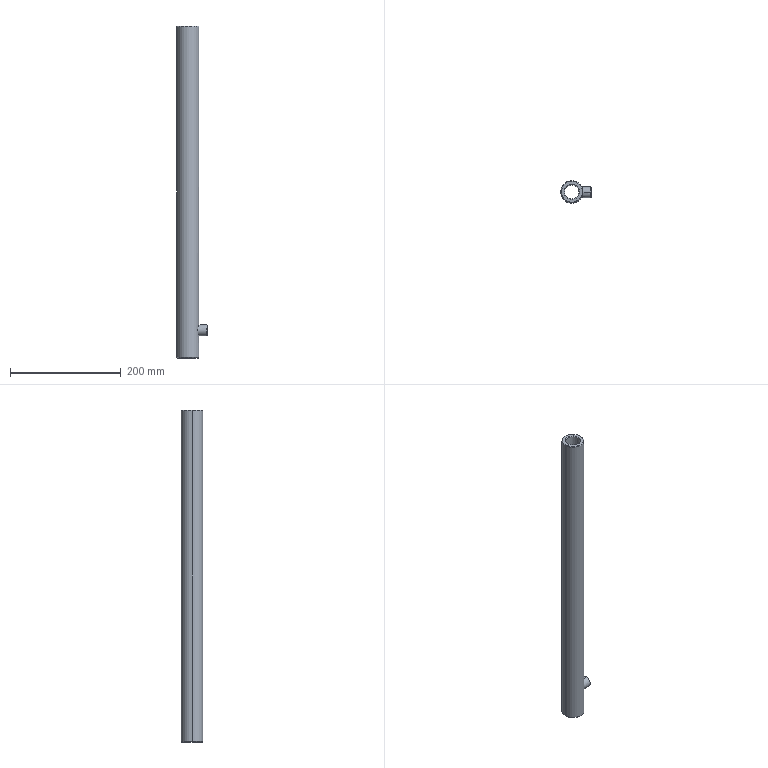Part | STEP file | Aluminium alloy sleeve | 1 solid | 21 faces | box 55 x 40 x 600 mm | volume 439299 mm3 | cone 10 | cylinder 8 | plane 3 | commonest cylinder face diameters 6.8 x2 20 x2 26 x2 40 x2